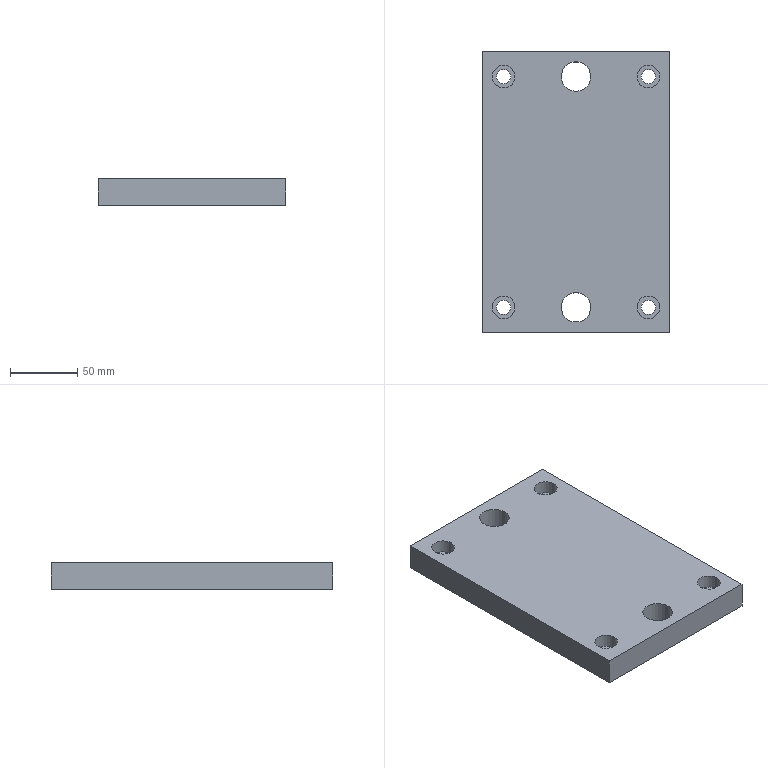Part | STEP file | 冲床-300配套压波_id1042_x_t | 1 solid | 20 faces | box 140 x 210 x 20 mm | volume 560119 mm3 | plane 10 | cylinder 10 | commonest cylinder face diameters 10.7 x4 17 x4 22 x2
STEP:
#1=CARTESIAN_POINT('',(1309.35,86.,289.));
#2=VERTEX_POINT('',#1);
#3=CARTESIAN_POINT('',(1304.,86.,289.));
#4=DIRECTION('',(0.,0.,1.));
#5=DIRECTION('',(1.,0.,0.));
#6=AXIS2_PLACEMENT_3D('',#3,#4,#5);
#7=CIRCLE('',#6,5.35);
#8=EDGE_CURVE('',#2,#2,#7,.T.);
#9=ORIENTED_EDGE('',*,*,#8,.F.);
#10=EDGE_LOOP('',(#9));
#11=FACE_BOUND('',#10,.T.);
#12=CARTESIAN_POINT('',(1312.5,86.,289.));
#13=VERTEX_POINT('',#12);
#14=CARTESIAN_POINT('',(1304.,86.,289.));
#15=DIRECTION('',(0.,0.,1.));
#16=DIRECTION('',(1.,0.,0.));
#17=AXIS2_PLACEMENT_3D('',#14,#15,#16);
#18=CIRCLE('',#17,8.5);
#19=EDGE_CURVE('',#13,#13,#18,.T.);
#20=ORIENTED_EDGE('',*,*,#19,.T.);
#21=EDGE_LOOP('',(#20));
#22=FACE_BOUND('',#21,.T.);
#23=CARTESIAN_POINT('',(1304.,86.,289.));
#24=DIRECTION('',(0.,0.,-1.));
#25=DIRECTION('',(1.,0.,0.));
#26=AXIS2_PLACEMENT_3D('',#23,#24,#25);
#27=PLANE('',#26);
#28=ADVANCED_FACE('',(#11,#22),#27,.F.);
#29=ORIENTED_EDGE('',*,*,#19,.F.);
#30=EDGE_LOOP('',(#29));
#31=FACE_BOUND('',#30,.T.);
#32=CARTESIAN_POINT('',(1312.5,86.,299.));
#33=VERTEX_POINT('',#32);
#34=CARTESIAN_POINT('',(1304.,86.,299.));
#35=DIRECTION('',(0.,0.,-1.));
#36=DIRECTION('',(1.,0.,0.));
#37=AXIS2_PLACEMENT_3D('',#34,#35,#36);
#38=CIRCLE('',#37,8.5);
#39=EDGE_CURVE('',#33,#33,#38,.T.);
#40=ORIENTED_EDGE('',*,*,#39,.F.);
#41=EDGE_LOOP('',(#40));
#42=FACE_BOUND('',#41,.T.);
#43=CARTESIAN_POINT('',(1304.,86.,299.));
#44=DIRECTION('',(0.,0.,-1.));
#45=DIRECTION('',(1.,0.,0.));
#46=AXIS2_PLACEMENT_3D('',#43,#44,#45);
#47=CYLINDRICAL_SURFACE('',#46,8.5);
#48=ADVANCED_FACE('',(#31,#42),#47,.F.);
#49=ORIENTED_EDGE('',*,*,#8,.T.);
#50=EDGE_LOOP('',(#49));
#51=FACE_BOUND('',#50,.T.);
#52=CARTESIAN_POINT('',(1298.65,86.,279.));
#53=VERTEX_POINT('',#52);
#54=CARTESIAN_POINT('',(1304.,86.,279.));
#55=DIRECTION('',(0.,0.,1.));
#56=DIRECTION('',(-1.,0.,0.));
#57=AXIS2_PLACEMENT_3D('',#54,#55,#56);
#58=CIRCLE('',#57,5.35);
#59=EDGE_CURVE('',#53,#53,#58,.T.);
#60=ORIENTED_EDGE('',*,*,#59,.F.);
#61=EDGE_LOOP('',(#60));
#62=FACE_BOUND('',#61,.T.);
#63=CARTESIAN_POINT('',(1304.,86.,196.873));
#64=DIRECTION('',(0.,0.,-1.));
#65=DIRECTION('',(1.,0.,0.));
#66=AXIS2_PLACEMENT_3D('',#63,#64,#65);
#67=CYLINDRICAL_SURFACE('',#66,5.35);
#68=ADVANCED_FACE('',(#51,#62),#67,.F.);
#69=CARTESIAN_POINT('',(1190.65,-86.,289.));
#70=VERTEX_POINT('',#69);
#71=CARTESIAN_POINT('',(1196.,-86.,289.));
#72=DIRECTION('',(0.,0.,1.));
#73=DIRECTION('',(-1.,0.,0.));
#74=AXIS2_PLACEMENT_3D('',#71,#72,#73);
#75=CIRCLE('',#74,5.35);
#76=EDGE_CURVE('',#70,#70,#75,.T.);
#77=ORIENTED_EDGE('',*,*,#76,.F.);
#78=EDGE_LOOP('',(#77));
#79=FACE_BOUND('',#78,.T.);
#80=CARTESIAN_POINT('',(1187.5,-86.,289.));
#81=VERTEX_POINT('',#80);
#82=CARTESIAN_POINT('',(1196.,-86.,289.));
#83=DIRECTION('',(0.,0.,1.));
#84=DIRECTION('',(-1.,0.,0.));
#85=AXIS2_PLACEMENT_3D('',#82,#83,#84);
#86=CIRCLE('',#85,8.5);
#87=EDGE_CURVE('',#81,#81,#86,.T.);
#88=ORIENTED_EDGE('',*,*,#87,.T.);
#89=EDGE_LOOP('',(#88));
#90=FACE_BOUND('',#89,.T.);
#91=CARTESIAN_POINT('',(1196.,-86.,289.));
#92=DIRECTION('',(0.,0.,-1.));
#93=DIRECTION('',(-1.,0.,0.));
#94=AXIS2_PLACEMENT_3D('',#91,#92,#93);
#95=PLANE('',#94);
#96=ADVANCED_FACE('',(#79,#90),#95,.F.);
#97=CARTESIAN_POINT('',(1190.65,86.,289.));
#98=VERTEX_POINT('',#97);
#99=CARTESIAN_POINT('',(1196.,86.,289.));
#100=DIRECTION('',(0.,0.,1.));
#101=DIRECTION('',(-1.,0.,0.));
#102=AXIS2_PLACEMENT_3D('',#99,#100,#101);
#103=CIRCLE('',#102,5.35);
#104=EDGE_CURVE('',#98,#98,#103,.T.);
#105=ORIENTED_EDGE('',*,*,#104,.F.);
#106=EDGE_LOOP('',(#105));
#107=FACE_BOUND('',#106,.T.);
#108=CARTESIAN_POINT('',(1187.5,86.,289.));
#109=VERTEX_POINT('',#108);
#110=CARTESIAN_POINT('',(1196.,86.,289.));
#111=DIRECTION('',(0.,0.,1.));
#112=DIRECTION('',(-1.,0.,0.));
#113=AXIS2_PLACEMENT_3D('',#110,#111,#112);
#114=CIRCLE('',#113,8.5);
#115=EDGE_CURVE('',#109,#109,#114,.T.);
#116=ORIENTED_EDGE('',*,*,#115,.T.);
#117=EDGE_LOOP('',(#116));
#118=FACE_BOUND('',#117,.T.);
#119=CARTESIAN_POINT('',(1196.,86.,289.));
#120=DIRECTION('',(0.,0.,-1.));
#121=DIRECTION('',(-1.,0.,0.));
#122=AXIS2_PLACEMENT_3D('',#119,#120,#121);
#123=PLANE('',#122);
#124=ADVANCED_FACE('',(#107,#118),#123,.F.);
#125=ORIENTED_EDGE('',*,*,#76,.T.);
#126=EDGE_LOOP('',(#125));
#127=FACE_BOUND('',#126,.T.);
#128=CARTESIAN_POINT('',(1201.35,-86.,279.));
#129=VERTEX_POINT('',#128);
#130=CARTESIAN_POINT('',(1196.,-86.,279.));
#131=DIRECTION('',(0.,0.,1.));
#132=DIRECTION('',(1.,0.,0.));
#133=AXIS2_PLACEMENT_3D('',#130,#131,#132);
#134=CIRCLE('',#133,5.35);
#135=EDGE_CURVE('',#129,#129,#134,.T.);
#136=ORIENTED_EDGE('',*,*,#135,.F.);
#137=EDGE_LOOP('',(#136));
#138=FACE_BOUND('',#137,.T.);
#139=CARTESIAN_POINT('',(1196.,-86.,196.873));
#140=DIRECTION('',(0.,0.,-1.));
#141=DIRECTION('',(-1.,0.,0.));
#142=AXIS2_PLACEMENT_3D('',#139,#140,#141);
#143=CYLINDRICAL_SURFACE('',#142,5.35);
#144=ADVANCED_FACE('',(#127,#138),#143,.F.);
#145=CARTESIAN_POINT('',(1180.,-105.,299.));
#146=VERTEX_POINT('',#145);
#147=CARTESIAN_POINT('',(1320.,-105.,299.));
#148=VERTEX_POINT('',#147);
#149=CARTESIAN_POINT('',(1190.,-105.,299.));
#150=DIRECTION('',(1.,0.,0.));
#151=VECTOR('',#150,1.);
#152=LINE('',#149,#151);
#153=EDGE_CURVE('',#146,#148,#152,.T.);
#154=ORIENTED_EDGE('',*,*,#153,.F.);
#155=CARTESIAN_POINT('',(1180.,-105.,279.));
#156=VERTEX_POINT('',#155);
#157=CARTESIAN_POINT('',(1180.,-105.,29.7));
#158=DIRECTION('',(0.,0.,1.));
#159=VECTOR('',#158,1.);
#160=LINE('',#157,#159);
#161=EDGE_CURVE('',#156,#146,#160,.T.);
#162=ORIENTED_EDGE('',*,*,#161,.F.);
#163=CARTESIAN_POINT('',(1320.,-105.,279.));
#164=VERTEX_POINT('',#163);
#165=CARTESIAN_POINT('',(1190.,-105.,279.));
#166=DIRECTION('',(1.,0.,0.));
#167=VECTOR('',#166,1.);
#168=LINE('',#165,#167);
#169=EDGE_CURVE('',#156,#164,#168,.T.);
#170=ORIENTED_EDGE('',*,*,#169,.T.);
#171=CARTESIAN_POINT('',(1320.,-105.,279.));
#172=DIRECTION('',(0.,0.,1.));
#173=VECTOR('',#172,1.);
#174=LINE('',#171,#173);
#175=EDGE_CURVE('',#164,#148,#174,.T.);
#176=ORIENTED_EDGE('',*,*,#175,.T.);
#177=EDGE_LOOP('',(#154,#162,#170,#176));
#178=FACE_OUTER_BOUND('',#177,.T.);
#179=CARTESIAN_POINT('',(1190.,-105.,279.));
#180=DIRECTION('',(0.,-1.,0.));
#181=DIRECTION('',(1.,0.,0.));
#182=AXIS2_PLACEMENT_3D('',#179,#180,#181);
#183=PLANE('',#182);
#184=ADVANCED_FACE('',(#178),#183,.T.);
#185=CARTESIAN_POINT('',(1180.,105.,299.));
#186=VERTEX_POINT('',#185);
#187=CARTESIAN_POINT('',(1180.,-140.,299.));
#188=DIRECTION('',(0.,-1.,0.));
#189=VECTOR('',#188,1.);
#190=LINE('',#187,#189);
#191=EDGE_CURVE('',#186,#146,#190,.T.);
#192=ORIENTED_EDGE('',*,*,#191,.F.);
#193=CARTESIAN_POINT('',(1180.,105.,279.));
#194=VERTEX_POINT('',#193);
#195=CARTESIAN_POINT('',(1180.,105.,279.));
#196=DIRECTION('',(0.,0.,1.));
#197=VECTOR('',#196,1.);
#198=LINE('',#195,#197);
#199=EDGE_CURVE('',#194,#186,#198,.T.);
#200=ORIENTED_EDGE('',*,*,#199,.F.);
#201=CARTESIAN_POINT('',(1180.,-140.,279.));
#202=DIRECTION('',(0.,-1.,0.));
#203=VECTOR('',#202,1.);
#204=LINE('',#201,#203);
#205=EDGE_CURVE('',#194,#156,#204,.T.);
#206=ORIENTED_EDGE('',*,*,#205,.T.);
#207=ORIENTED_EDGE('',*,*,#161,.T.);
#208=EDGE_LOOP('',(#192,#200,#206,#207));
#209=FACE_OUTER_BOUND('',#208,.T.);
#210=CARTESIAN_POINT('',(1180.,-71.,29.7));
#211=DIRECTION('',(1.,0.,0.));
#212=DIRECTION('',(0.,0.,1.));
#213=AXIS2_PLACEMENT_3D('',#210,#211,#212);
#214=PLANE('',#213);
#215=ADVANCED_FACE('',(#209),#214,.F.);
#216=CARTESIAN_POINT('',(1320.,105.,299.));
#217=VERTEX_POINT('',#216);
#218=CARTESIAN_POINT('',(1190.,105.,299.));
#219=DIRECTION('',(-1.,0.,0.));
#220=VECTOR('',#219,1.);
#221=LINE('',#218,#220);
#222=EDGE_CURVE('',#217,#186,#221,.T.);
#223=ORIENTED_EDGE('',*,*,#222,.F.);
#224=CARTESIAN_POINT('',(1320.,105.,279.));
#225=VERTEX_POINT('',#224);
#226=CARTESIAN_POINT('',(1320.,105.,29.7));
#227=DIRECTION('',(0.,0.,1.));
#228=VECTOR('',#227,1.);
#229=LINE('',#226,#228);
#230=EDGE_CURVE('',#225,#217,#229,.T.);
#231=ORIENTED_EDGE('',*,*,#230,.F.);
#232=CARTESIAN_POINT('',(1190.,105.,279.));
#233=DIRECTION('',(-1.,0.,0.));
#234=VECTOR('',#233,1.);
#235=LINE('',#232,#234);
#236=EDGE_CURVE('',#225,#194,#235,.T.);
#237=ORIENTED_EDGE('',*,*,#236,.T.);
#238=ORIENTED_EDGE('',*,*,#199,.T.);
#239=EDGE_LOOP('',(#223,#231,#237,#238));
#240=FACE_OUTER_BOUND('',#239,.T.);
#241=CARTESIAN_POINT('',(1310.,105.,279.));
#242=DIRECTION('',(0.,1.,0.));
#243=DIRECTION('',(-1.,0.,0.));
#244=AXIS2_PLACEMENT_3D('',#241,#242,#243);
#245=PLANE('',#244);
#246=ADVANCED_FACE('',(#240),#245,.T.);
#247=CARTESIAN_POINT('',(1320.,-140.,299.));
#248=DIRECTION('',(0.,1.,0.));
#249=VECTOR('',#248,1.);
#250=LINE('',#247,#249);
#251=EDGE_CURVE('',#148,#217,#250,.T.);
#252=ORIENTED_EDGE('',*,*,#251,.F.);
#253=ORIENTED_EDGE('',*,*,#175,.F.);
#254=CARTESIAN_POINT('',(1320.,-140.,279.));
#255=DIRECTION('',(0.,1.,0.));
#256=VECTOR('',#255,1.);
#257=LINE('',#254,#256);
#258=EDGE_CURVE('',#164,#225,#257,.T.);
#259=ORIENTED_EDGE('',*,*,#258,.T.);
#260=ORIENTED_EDGE('',*,*,#230,.T.);
#261=EDGE_LOOP('',(#252,#253,#259,#260));
#262=FACE_OUTER_BOUND('',#261,.T.);
#263=CARTESIAN_POINT('',(1320.,-71.,29.7));
#264=DIRECTION('',(-1.,0.,0.));
#265=DIRECTION('',(0.,0.,1.));
#266=AXIS2_PLACEMENT_3D('',#263,#264,#265);
#267=PLANE('',#266);
#268=ADVANCED_FACE('',(#262),#267,.F.);
#269=CARTESIAN_POINT('',(1261.,-86.,299.));
#270=VERTEX_POINT('',#269);
#271=CARTESIAN_POINT('',(1250.,-86.,299.));
#272=DIRECTION('',(0.,0.,-1.));
#273=DIRECTION('',(1.,0.,0.));
#274=AXIS2_PLACEMENT_3D('',#271,#272,#273);
#275=CIRCLE('',#274,11.);
#276=EDGE_CURVE('',#270,#270,#275,.T.);
#277=ORIENTED_EDGE('',*,*,#276,.F.);
#278=EDGE_LOOP('',(#277));
#279=FACE_BOUND('',#278,.T.);
#280=CARTESIAN_POINT('',(1261.,-86.,279.));
#281=VERTEX_POINT('',#280);
#282=CARTESIAN_POINT('',(1250.,-86.,279.));
#283=DIRECTION('',(0.,0.,1.));
#284=DIRECTION('',(1.,0.,0.));
#285=AXIS2_PLACEMENT_3D('',#282,#283,#284);
#286=CIRCLE('',#285,11.);
#287=EDGE_CURVE('',#281,#281,#286,.T.);
#288=ORIENTED_EDGE('',*,*,#287,.F.);
#289=EDGE_LOOP('',(#288));
#290=FACE_BOUND('',#289,.T.);
#291=CARTESIAN_POINT('',(1250.,-86.,299.));
#292=DIRECTION('',(0.,0.,-1.));
#293=DIRECTION('',(-1.,0.,0.));
#294=AXIS2_PLACEMENT_3D('',#291,#292,#293);
#295=CYLINDRICAL_SURFACE('',#294,11.);
#296=ADVANCED_FACE('',(#279,#290),#295,.F.);
#297=ORIENTED_EDGE('',*,*,#87,.F.);
#298=EDGE_LOOP('',(#297));
#299=FACE_BOUND('',#298,.T.);
#300=CARTESIAN_POINT('',(1187.5,-86.,299.));
#301=VERTEX_POINT('',#300);
#302=CARTESIAN_POINT('',(1196.,-86.,299.));
#303=DIRECTION('',(0.,0.,-1.));
#304=DIRECTION('',(-1.,0.,0.));
#305=AXIS2_PLACEMENT_3D('',#302,#303,#304);
#306=CIRCLE('',#305,8.5);
#307=EDGE_CURVE('',#301,#301,#306,.T.);
#308=ORIENTED_EDGE('',*,*,#307,.F.);
#309=EDGE_LOOP('',(#308));
#310=FACE_BOUND('',#309,.T.);
#311=CARTESIAN_POINT('',(1196.,-86.,299.));
#312=DIRECTION('',(0.,0.,-1.));
#313=DIRECTION('',(-1.,0.,0.));
#314=AXIS2_PLACEMENT_3D('',#311,#312,#313);
#315=CYLINDRICAL_SURFACE('',#314,8.5);
#316=ADVANCED_FACE('',(#299,#310),#315,.F.);
#317=CARTESIAN_POINT('',(1261.,86.,299.));
#318=VERTEX_POINT('',#317);
#319=CARTESIAN_POINT('',(1250.,86.,299.));
#320=DIRECTION('',(0.,0.,-1.));
#321=DIRECTION('',(1.,0.,0.));
#322=AXIS2_PLACEMENT_3D('',#319,#320,#321);
#323=CIRCLE('',#322,11.);
#324=EDGE_CURVE('',#318,#318,#323,.T.);
#325=ORIENTED_EDGE('',*,*,#324,.F.);
#326=EDGE_LOOP('',(#325));
#327=FACE_BOUND('',#326,.T.);
#328=CARTESIAN_POINT('',(1261.,86.,279.));
#329=VERTEX_POINT('',#328);
#330=CARTESIAN_POINT('',(1250.,86.,279.));
#331=DIRECTION('',(0.,0.,1.));
#332=DIRECTION('',(1.,0.,0.));
#333=AXIS2_PLACEMENT_3D('',#330,#331,#332);
#334=CIRCLE('',#333,11.);
#335=EDGE_CURVE('',#329,#329,#334,.T.);
#336=ORIENTED_EDGE('',*,*,#335,.F.);
#337=EDGE_LOOP('',(#336));
#338=FACE_BOUND('',#337,.T.);
#339=CARTESIAN_POINT('',(1250.,86.,299.));
#340=DIRECTION('',(0.,0.,-1.));
#341=DIRECTION('',(-1.,0.,0.));
#342=AXIS2_PLACEMENT_3D('',#339,#340,#341);
#343=CYLINDRICAL_SURFACE('',#342,11.);
#344=ADVANCED_FACE('',(#327,#338),#343,.F.);
#345=ORIENTED_EDGE('',*,*,#115,.F.);
#346=EDGE_LOOP('',(#345));
#347=FACE_BOUND('',#346,.T.);
#348=CARTESIAN_POINT('',(1187.5,86.,299.));
#349=VERTEX_POINT('',#348);
#350=CARTESIAN_POINT('',(1196.,86.,299.));
#351=DIRECTION('',(0.,0.,-1.));
#352=DIRECTION('',(-1.,0.,0.));
#353=AXIS2_PLACEMENT_3D('',#350,#351,#352);
#354=CIRCLE('',#353,8.5);
#355=EDGE_CURVE('',#349,#349,#354,.T.);
#356=ORIENTED_EDGE('',*,*,#355,.F.);
#357=EDGE_LOOP('',(#356));
#358=FACE_BOUND('',#357,.T.);
#359=CARTESIAN_POINT('',(1196.,86.,299.));
#360=DIRECTION('',(0.,0.,-1.));
#361=DIRECTION('',(-1.,0.,0.));
#362=AXIS2_PLACEMENT_3D('',#359,#360,#361);
#363=CYLINDRICAL_SURFACE('',#362,8.5);
#364=ADVANCED_FACE('',(#347,#358),#363,.F.);
#365=CARTESIAN_POINT('',(1312.5,-86.,299.));
#366=VERTEX_POINT('',#365);
#367=CARTESIAN_POINT('',(1304.,-86.,299.));
#368=DIRECTION('',(0.,0.,-1.));
#369=DIRECTION('',(1.,0.,0.));
#370=AXIS2_PLACEMENT_3D('',#367,#368,#369);
#371=CIRCLE('',#370,8.5);
#372=EDGE_CURVE('',#366,#366,#371,.T.);
#373=ORIENTED_EDGE('',*,*,#372,.T.);
#374=EDGE_LOOP('',(#373));
#375=FACE_BOUND('',#374,.T.);
#376=ORIENTED_EDGE('',*,*,#39,.T.);
#377=EDGE_LOOP('',(#376));
#378=FACE_BOUND('',#377,.T.);
#379=ORIENTED_EDGE('',*,*,#355,.T.);
#380=EDGE_LOOP('',(#379));
#381=FACE_BOUND('',#380,.T.);
#382=ORIENTED_EDGE('',*,*,#324,.T.);
#383=EDGE_LOOP('',(#382));
#384=FACE_BOUND('',#383,.T.);
#385=ORIENTED_EDGE('',*,*,#307,.T.);
#386=EDGE_LOOP('',(#385));
#387=FACE_BOUND('',#386,.T.);
#388=ORIENTED_EDGE('',*,*,#276,.T.);
#389=EDGE_LOOP('',(#388));
#390=FACE_BOUND('',#389,.T.);
#391=ORIENTED_EDGE('',*,*,#251,.T.);
#392=ORIENTED_EDGE('',*,*,#222,.T.);
#393=ORIENTED_EDGE('',*,*,#191,.T.);
#394=ORIENTED_EDGE('',*,*,#153,.T.);
#395=EDGE_LOOP('',(#391,#392,#393,#394));
#396=FACE_BOUND('',#395,.T.);
#397=CARTESIAN_POINT('',(1190.,-140.,299.));
#398=DIRECTION('',(0.,0.,1.));
#399=DIRECTION('',(1.,0.,0.));
#400=AXIS2_PLACEMENT_3D('',#397,#398,#399);
#401=PLANE('',#400);
#402=ADVANCED_FACE('',(#375,#378,#381,#384,#387,#390,#396),#401,.T.);
#403=ORIENTED_EDGE('',*,*,#104,.T.);
#404=EDGE_LOOP('',(#403));
#405=FACE_BOUND('',#404,.T.);
#406=CARTESIAN_POINT('',(1201.35,86.,279.));
#407=VERTEX_POINT('',#406);
#408=CARTESIAN_POINT('',(1196.,86.,279.));
#409=DIRECTION('',(0.,0.,1.));
#410=DIRECTION('',(1.,0.,0.));
#411=AXIS2_PLACEMENT_3D('',#408,#409,#410);
#412=CIRCLE('',#411,5.35);
#413=EDGE_CURVE('',#407,#407,#412,.T.);
#414=ORIENTED_EDGE('',*,*,#413,.F.);
#415=EDGE_LOOP('',(#414));
#416=FACE_BOUND('',#415,.T.);
#417=CARTESIAN_POINT('',(1196.,86.,196.873));
#418=DIRECTION('',(0.,0.,-1.));
#419=DIRECTION('',(-1.,0.,0.));
#420=AXIS2_PLACEMENT_3D('',#417,#418,#419);
#421=CYLINDRICAL_SURFACE('',#420,5.35);
#422=ADVANCED_FACE('',(#405,#416),#421,.F.);
#423=CARTESIAN_POINT('',(1298.65,-86.,279.));
#424=VERTEX_POINT('',#423);
#425=CARTESIAN_POINT('',(1304.,-86.,279.));
#426=DIRECTION('',(0.,0.,1.));
#427=DIRECTION('',(-1.,0.,0.));
#428=AXIS2_PLACEMENT_3D('',#425,#426,#427);
#429=CIRCLE('',#428,5.35);
#430=EDGE_CURVE('',#424,#424,#429,.T.);
#431=ORIENTED_EDGE('',*,*,#430,.T.);
#432=EDGE_LOOP('',(#431));
#433=FACE_BOUND('',#432,.T.);
#434=ORIENTED_EDGE('',*,*,#59,.T.);
#435=EDGE_LOOP('',(#434));
#436=FACE_BOUND('',#435,.T.);
#437=ORIENTED_EDGE('',*,*,#413,.T.);
#438=EDGE_LOOP('',(#437));
#439=FACE_BOUND('',#438,.T.);
#440=ORIENTED_EDGE('',*,*,#335,.T.);
#441=EDGE_LOOP('',(#440));
#442=FACE_BOUND('',#441,.T.);
#443=ORIENTED_EDGE('',*,*,#135,.T.);
#444=EDGE_LOOP('',(#443));
#445=FACE_BOUND('',#444,.T.);
#446=ORIENTED_EDGE('',*,*,#287,.T.);
#447=EDGE_LOOP('',(#446));
#448=FACE_BOUND('',#447,.T.);
#449=ORIENTED_EDGE('',*,*,#258,.F.);
#450=ORIENTED_EDGE('',*,*,#169,.F.);
#451=ORIENTED_EDGE('',*,*,#205,.F.);
#452=ORIENTED_EDGE('',*,*,#236,.F.);
#453=EDGE_LOOP('',(#449,#450,#451,#452));
#454=FACE_BOUND('',#453,.T.);
#455=CARTESIAN_POINT('',(1190.,-140.,279.));
#456=DIRECTION('',(0.,0.,1.));
#457=DIRECTION('',(1.,0.,0.));
#458=AXIS2_PLACEMENT_3D('',#455,#456,#457);
#459=PLANE('',#458);
#460=ADVANCED_FACE('',(#433,#436,#439,#442,#445,#448,#454),#459,.F.);
#461=CARTESIAN_POINT('',(1309.35,-86.,289.));
#462=VERTEX_POINT('',#461);
#463=CARTESIAN_POINT('',(1304.,-86.,289.));
#464=DIRECTION('',(0.,0.,1.));
#465=DIRECTION('',(1.,0.,0.));
#466=AXIS2_PLACEMENT_3D('',#463,#464,#465);
#467=CIRCLE('',#466,5.35);
#468=EDGE_CURVE('',#462,#462,#467,.T.);
#469=ORIENTED_EDGE('',*,*,#468,.F.);
#470=EDGE_LOOP('',(#469));
#471=FACE_BOUND('',#470,.T.);
#472=CARTESIAN_POINT('',(1312.5,-86.,289.));
#473=VERTEX_POINT('',#472);
#474=CARTESIAN_POINT('',(1304.,-86.,289.));
#475=DIRECTION('',(0.,0.,1.));
#476=DIRECTION('',(1.,0.,0.));
#477=AXIS2_PLACEMENT_3D('',#474,#475,#476);
#478=CIRCLE('',#477,8.5);
#479=EDGE_CURVE('',#473,#473,#478,.T.);
#480=ORIENTED_EDGE('',*,*,#479,.T.);
#481=EDGE_LOOP('',(#480));
#482=FACE_BOUND('',#481,.T.);
#483=CARTESIAN_POINT('',(1304.,-86.,289.));
#484=DIRECTION('',(0.,0.,-1.));
#485=DIRECTION('',(1.,0.,0.));
#486=AXIS2_PLACEMENT_3D('',#483,#484,#485);
#487=PLANE('',#486);
#488=ADVANCED_FACE('',(#471,#482),#487,.F.);
#489=ORIENTED_EDGE('',*,*,#479,.F.);
#490=EDGE_LOOP('',(#489));
#491=FACE_BOUND('',#490,.T.);
#492=ORIENTED_EDGE('',*,*,#372,.F.);
#493=EDGE_LOOP('',(#492));
#494=FACE_BOUND('',#493,.T.);
#495=CARTESIAN_POINT('',(1304.,-86.,299.));
#496=DIRECTION('',(0.,0.,-1.));
#497=DIRECTION('',(1.,0.,0.));
#498=AXIS2_PLACEMENT_3D('',#495,#496,#497);
#499=CYLINDRICAL_SURFACE('',#498,8.5);
#500=ADVANCED_FACE('',(#491,#494),#499,.F.);
#501=ORIENTED_EDGE('',*,*,#468,.T.);
#502=EDGE_LOOP('',(#501));
#503=FACE_BOUND('',#502,.T.);
#504=ORIENTED_EDGE('',*,*,#430,.F.);
#505=EDGE_LOOP('',(#504));
#506=FACE_BOUND('',#505,.T.);
#507=CARTESIAN_POINT('',(1304.,-86.,196.873));
#508=DIRECTION('',(0.,0.,-1.));
#509=DIRECTION('',(1.,0.,0.));
#510=AXIS2_PLACEMENT_3D('',#507,#508,#509);
#511=CYLINDRICAL_SURFACE('',#510,5.35);
#512=ADVANCED_FACE('',(#503,#506),#511,.F.);
#513=CLOSED_SHELL('',(#28,#48,#68,#96,#124,#144,#184,#215,#246,#268,#296,#316,#344,#364,#402,#422,#460,#488,#500,#512));
#514=MANIFOLD_SOLID_BREP('',#513);
#515=(LENGTH_UNIT()NAMED_UNIT(*)SI_UNIT(.MILLI.,.METRE.));
#516=UNCERTAINTY_MEASURE_WITH_UNIT(LENGTH_MEASURE(0.00002),#515,'','');
#517=(NAMED_UNIT(*)PLANE_ANGLE_UNIT()SI_UNIT($,.RADIAN.));
#518=PLANE_ANGLE_MEASURE_WITH_UNIT(PLANE_ANGLE_MEASURE(0.01745),#517);
#519=DIMENSIONAL_EXPONENTS(0.,0.,0.,0.,0.,0.,0.);
#520=(CONVERSION_BASED_UNIT('DEGREE',#518)NAMED_UNIT(#519)PLANE_ANGLE_UNIT());
#521=(NAMED_UNIT(*)SI_UNIT($,.STERADIAN.)SOLID_ANGLE_UNIT());
#522=(GEOMETRIC_REPRESENTATION_CONTEXT(3)GLOBAL_UNCERTAINTY_ASSIGNED_CONTEXT((#516))GLOBAL_UNIT_ASSIGNED_CONTEXT((#515,#520,#521))REPRESENTATION_CONTEXT('',''));
#523=ADVANCED_BREP_SHAPE_REPRESENTATION('',(#514),#522);